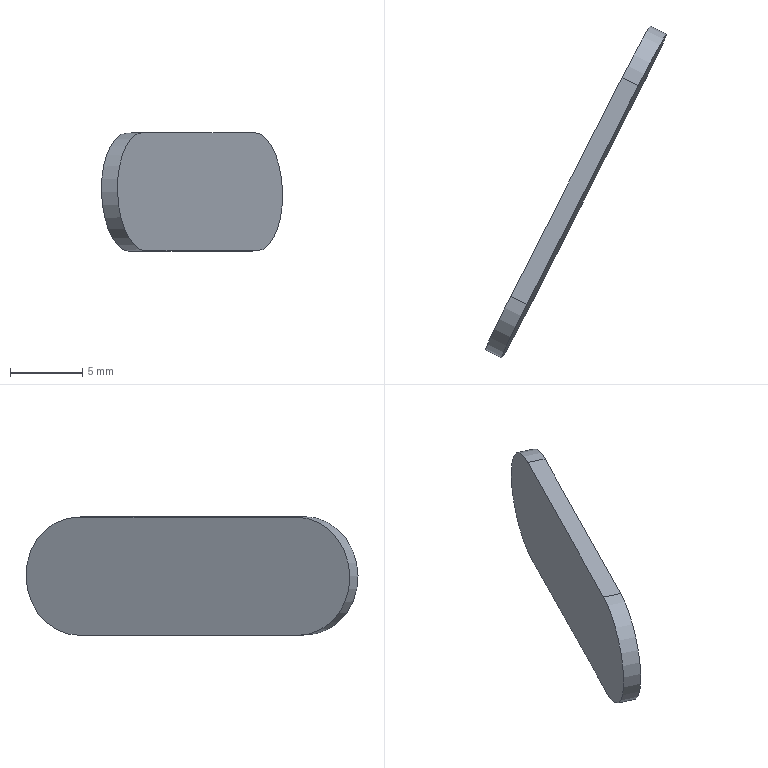Part | STEP file | 9805823280.1BPIECE_SOLIDE_FINALE_id1758_x_t | 1 solid | 6 faces | box 12.56 x 23.021 x 8.234 mm | volume 240.263 mm3 | plane 4 | cylinder 2 | commonest cylinder face diameters 8.2 x2
STEP:
#1=CARTESIAN_POINT('',(0.,0.,0.));
#2=DIRECTION('',(0.,0.,1.));
#3=DIRECTION('',(1.,0.,0.));
#4=AXIS2_PLACEMENT_3D('',#1,#2,#3);
#5=CARTESIAN_POINT('',(1096.718,-7.794,-24.025));
#6=VERTEX_POINT('',#5);
#7=CARTESIAN_POINT('',(1089.,-22.942,-24.025));
#8=VERTEX_POINT('',#7);
#9=CARTESIAN_POINT('',(1092.859,-15.368,-24.025));
#10=DIRECTION('',(-0.454,-0.891,0.));
#11=VECTOR('',#10,1.);
#12=LINE('',#9,#11);
#13=CARTESIAN_POINT('',(1077.019,-59.966,-230.062));
#14=DIRECTION('',(-0.8906,0.4538,-0.02975));
#15=DIRECTION('',(-0.02651,0.01351,0.9996));
#16=AXIS2_PLACEMENT_3D('',#13,#14,#15);
#17=PLANE('',#16);
#18=CARTESIAN_POINT('',(206.129,46.928));
#19=DIRECTION('',(0.000000001,-1.));
#20=VECTOR('',#19,1.);
#21=LINE('',#18,#20);
#22=(GEOMETRIC_REPRESENTATION_CONTEXT(2)PARAMETRIC_REPRESENTATION_CONTEXT()REPRESENTATION_CONTEXT('',''));
#23=DEFINITIONAL_REPRESENTATION('',(#21),#22);
#24=PCURVE('',#17,#23);
#25=CARTESIAN_POINT('',(1097.831,-8.362,-23.988));
#26=DIRECTION('',(0.02651,-0.01351,-0.9996));
#27=DIRECTION('',(0.454,0.891,0.));
#28=AXIS2_PLACEMENT_3D('',#25,#26,#27);
#29=PLANE('',#28);
#30=CARTESIAN_POINT('',(-8.5,-1.25));
#31=DIRECTION('',(-1.,0.));
#32=VECTOR('',#31,1.);
#33=LINE('',#30,#32);
#34=(GEOMETRIC_REPRESENTATION_CONTEXT(2)PARAMETRIC_REPRESENTATION_CONTEXT()REPRESENTATION_CONTEXT('',''));
#35=DEFINITIONAL_REPRESENTATION('',(#33),#34);
#36=PCURVE('',#29,#35);
#37=SURFACE_CURVE('',#12,(#24,#36),.PCURVE_S1.);
#38=EDGE_CURVE('',#6,#8,#37,.T.);
#39=ORIENTED_EDGE('',*,*,#38,.T.);
#40=CARTESIAN_POINT('',(1088.783,-22.831,-15.828));
#41=VERTEX_POINT('',#40);
#42=CARTESIAN_POINT('',(1088.892,-22.886,-19.927));
#43=DIRECTION('',(-0.8906,0.4538,-0.02975));
#44=DIRECTION('',(-0.02651,0.01351,0.9996));
#45=AXIS2_PLACEMENT_3D('',#42,#43,#44);
#46=CIRCLE('',#45,4.1);
#47=CARTESIAN_POINT('',(210.229,38.428));
#48=DIRECTION('',(1.,0.000000001));
#49=AXIS2_PLACEMENT_2D('',#47,#48);
#50=CIRCLE('',#49,4.1);
#51=(GEOMETRIC_REPRESENTATION_CONTEXT(2)PARAMETRIC_REPRESENTATION_CONTEXT()REPRESENTATION_CONTEXT('',''));
#52=DEFINITIONAL_REPRESENTATION('',(#50),#51);
#53=PCURVE('',#17,#52);
#54=CARTESIAN_POINT('',(1090.005,-23.453,-19.889));
#55=DIRECTION('',(0.8906,-0.4538,0.02975));
#56=DIRECTION('',(0.02651,-0.01351,-0.9996));
#57=AXIS2_PLACEMENT_3D('',#54,#55,#56);
#58=CYLINDRICAL_SURFACE('',#57,4.1);
#59=CARTESIAN_POINT('',(9.425,-1.25));
#60=DIRECTION('',(-1.,0.));
#61=VECTOR('',#60,1.);
#62=LINE('',#59,#61);
#63=(GEOMETRIC_REPRESENTATION_CONTEXT(2)PARAMETRIC_REPRESENTATION_CONTEXT()REPRESENTATION_CONTEXT('',''));
#64=DEFINITIONAL_REPRESENTATION('',(#62),#63);
#65=PCURVE('',#58,#64);
#66=SURFACE_CURVE('',#46,(#53,#65),.PCURVE_S1.);
#67=EDGE_CURVE('',#8,#41,#66,.T.);
#68=ORIENTED_EDGE('',*,*,#67,.T.);
#69=CARTESIAN_POINT('',(1096.501,-7.684,-15.828));
#70=VERTEX_POINT('',#69);
#71=CARTESIAN_POINT('',(1092.642,-15.257,-15.828));
#72=DIRECTION('',(0.454,0.891,0.));
#73=VECTOR('',#72,1.);
#74=LINE('',#71,#73);
#75=CARTESIAN_POINT('',(214.329,46.928));
#76=DIRECTION('',(-0.000000001,1.));
#77=VECTOR('',#76,1.);
#78=LINE('',#75,#77);
#79=(GEOMETRIC_REPRESENTATION_CONTEXT(2)PARAMETRIC_REPRESENTATION_CONTEXT()REPRESENTATION_CONTEXT('',''));
#80=DEFINITIONAL_REPRESENTATION('',(#78),#79);
#81=PCURVE('',#17,#80);
#82=CARTESIAN_POINT('',(1089.896,-23.398,-15.791));
#83=DIRECTION('',(-0.02651,0.01351,0.9996));
#84=DIRECTION('',(-0.454,-0.891,0.));
#85=AXIS2_PLACEMENT_3D('',#82,#83,#84);
#86=PLANE('',#85);
#87=CARTESIAN_POINT('',(-8.5,-1.25));
#88=DIRECTION('',(-1.,0.));
#89=VECTOR('',#88,1.);
#90=LINE('',#87,#89);
#91=(GEOMETRIC_REPRESENTATION_CONTEXT(2)PARAMETRIC_REPRESENTATION_CONTEXT()REPRESENTATION_CONTEXT('',''));
#92=DEFINITIONAL_REPRESENTATION('',(#90),#91);
#93=PCURVE('',#86,#92);
#94=SURFACE_CURVE('',#74,(#81,#93),.PCURVE_S1.);
#95=EDGE_CURVE('',#41,#70,#94,.T.);
#96=ORIENTED_EDGE('',*,*,#95,.T.);
#97=CARTESIAN_POINT('',(1096.609,-7.739,-19.927));
#98=DIRECTION('',(-0.8906,0.4538,-0.02975));
#99=DIRECTION('',(-0.02651,0.01351,0.9996));
#100=AXIS2_PLACEMENT_3D('',#97,#98,#99);
#101=CIRCLE('',#100,4.1);
#102=CARTESIAN_POINT('',(210.229,55.428));
#103=DIRECTION('',(1.,0.000000001));
#104=AXIS2_PLACEMENT_2D('',#102,#103);
#105=CIRCLE('',#104,4.1);
#106=(GEOMETRIC_REPRESENTATION_CONTEXT(2)PARAMETRIC_REPRESENTATION_CONTEXT()REPRESENTATION_CONTEXT('',''));
#107=DEFINITIONAL_REPRESENTATION('',(#105),#106);
#108=PCURVE('',#17,#107);
#109=CARTESIAN_POINT('',(1097.723,-8.306,-19.889));
#110=DIRECTION('',(0.8906,-0.4538,0.02975));
#111=DIRECTION('',(-0.02651,0.01351,0.9996));
#112=AXIS2_PLACEMENT_3D('',#109,#110,#111);
#113=CYLINDRICAL_SURFACE('',#112,4.1);
#114=CARTESIAN_POINT('',(6.283,-1.25));
#115=DIRECTION('',(-1.,0.));
#116=VECTOR('',#115,1.);
#117=LINE('',#114,#116);
#118=(GEOMETRIC_REPRESENTATION_CONTEXT(2)PARAMETRIC_REPRESENTATION_CONTEXT()REPRESENTATION_CONTEXT('',''));
#119=DEFINITIONAL_REPRESENTATION('',(#117),#118);
#120=PCURVE('',#113,#119);
#121=SURFACE_CURVE('',#101,(#108,#120),.PCURVE_S1.);
#122=EDGE_CURVE('',#70,#6,#121,.T.);
#123=ORIENTED_EDGE('',*,*,#122,.T.);
#124=EDGE_LOOP('',(#39,#68,#96,#123));
#125=FACE_BOUND('',#124,.T.);
#126=ADVANCED_FACE('',(#125),#17,.T.);
#127=CARTESIAN_POINT('',(1090.113,-23.509,-23.988));
#128=VERTEX_POINT('',#127);
#129=CARTESIAN_POINT('',(1090.113,-23.509,-23.988));
#130=DIRECTION('',(0.8906,-0.4538,0.02975));
#131=VECTOR('',#130,1.);
#132=LINE('',#129,#131);
#133=CARTESIAN_POINT('',(6.283,0.));
#134=DIRECTION('',(0.,1.));
#135=VECTOR('',#134,1.);
#136=LINE('',#133,#135);
#137=(GEOMETRIC_REPRESENTATION_CONTEXT(2)PARAMETRIC_REPRESENTATION_CONTEXT()REPRESENTATION_CONTEXT('',''));
#138=DEFINITIONAL_REPRESENTATION('',(#136),#137);
#139=PCURVE('',#58,#138);
#140=CARTESIAN_POINT('',(-17.,0.));
#141=DIRECTION('',(0.,1.));
#142=VECTOR('',#141,1.);
#143=LINE('',#140,#142);
#144=(GEOMETRIC_REPRESENTATION_CONTEXT(2)PARAMETRIC_REPRESENTATION_CONTEXT()REPRESENTATION_CONTEXT('',''));
#145=DEFINITIONAL_REPRESENTATION('',(#143),#144);
#146=PCURVE('',#29,#145);
#147=SURFACE_CURVE('',#132,(#139,#146),.PCURVE_S1.);
#148=EDGE_CURVE('',#8,#128,#147,.T.);
#149=ORIENTED_EDGE('',*,*,#148,.T.);
#150=CARTESIAN_POINT('',(1089.896,-23.398,-15.791));
#151=VERTEX_POINT('',#150);
#152=CARTESIAN_POINT('',(1090.005,-23.453,-19.889));
#153=DIRECTION('',(-0.8906,0.4538,-0.02975));
#154=DIRECTION('',(-0.02651,0.01351,0.9996));
#155=AXIS2_PLACEMENT_3D('',#152,#153,#154);
#156=CIRCLE('',#155,4.1);
#157=CARTESIAN_POINT('',(9.425,0.));
#158=DIRECTION('',(-1.,0.));
#159=VECTOR('',#158,1.);
#160=LINE('',#157,#159);
#161=(GEOMETRIC_REPRESENTATION_CONTEXT(2)PARAMETRIC_REPRESENTATION_CONTEXT()REPRESENTATION_CONTEXT('',''));
#162=DEFINITIONAL_REPRESENTATION('',(#160),#161);
#163=PCURVE('',#58,#162);
#164=CARTESIAN_POINT('',(1078.132,-60.533,-230.025));
#165=DIRECTION('',(-0.8906,0.4538,-0.02975));
#166=DIRECTION('',(-0.02651,0.01351,0.9996));
#167=AXIS2_PLACEMENT_3D('',#164,#165,#166);
#168=PLANE('',#167);
#169=CARTESIAN_POINT('',(210.229,38.428));
#170=DIRECTION('',(1.,0.000000001));
#171=AXIS2_PLACEMENT_2D('',#169,#170);
#172=CIRCLE('',#171,4.1);
#173=(GEOMETRIC_REPRESENTATION_CONTEXT(2)PARAMETRIC_REPRESENTATION_CONTEXT()REPRESENTATION_CONTEXT('',''));
#174=DEFINITIONAL_REPRESENTATION('',(#172),#173);
#175=PCURVE('',#168,#174);
#176=SURFACE_CURVE('',#156,(#163,#175),.PCURVE_S1.);
#177=EDGE_CURVE('',#128,#151,#176,.T.);
#178=ORIENTED_EDGE('',*,*,#177,.T.);
#179=CARTESIAN_POINT('',(1089.896,-23.398,-15.791));
#180=DIRECTION('',(0.8906,-0.4538,0.02975));
#181=VECTOR('',#180,1.);
#182=LINE('',#179,#181);
#183=CARTESIAN_POINT('',(3.142,0.));
#184=DIRECTION('',(0.,1.));
#185=VECTOR('',#184,1.);
#186=LINE('',#183,#185);
#187=(GEOMETRIC_REPRESENTATION_CONTEXT(2)PARAMETRIC_REPRESENTATION_CONTEXT()REPRESENTATION_CONTEXT('',''));
#188=DEFINITIONAL_REPRESENTATION('',(#186),#187);
#189=PCURVE('',#58,#188);
#190=CARTESIAN_POINT('',(0.,0.));
#191=DIRECTION('',(0.,1.));
#192=VECTOR('',#191,1.);
#193=LINE('',#190,#192);
#194=(GEOMETRIC_REPRESENTATION_CONTEXT(2)PARAMETRIC_REPRESENTATION_CONTEXT()REPRESENTATION_CONTEXT('',''));
#195=DEFINITIONAL_REPRESENTATION('',(#193),#194);
#196=PCURVE('',#86,#195);
#197=SURFACE_CURVE('',#182,(#189,#196),.PCURVE_S1.);
#198=EDGE_CURVE('',#41,#151,#197,.T.);
#199=ORIENTED_EDGE('',*,*,#198,.F.);
#200=ORIENTED_EDGE('',*,*,#67,.F.);
#201=EDGE_LOOP('',(#149,#178,#199,#200));
#202=FACE_BOUND('',#201,.T.);
#203=ADVANCED_FACE('',(#202),#58,.T.);
#204=CARTESIAN_POINT('',(1097.831,-8.362,-23.988));
#205=VERTEX_POINT('',#204);
#206=CARTESIAN_POINT('',(1097.275,-8.078,-24.006));
#207=DIRECTION('',(0.8906,-0.4538,0.02975));
#208=VECTOR('',#207,1.);
#209=LINE('',#206,#208);
#210=CARTESIAN_POINT('',(0.,-0.625));
#211=DIRECTION('',(0.,1.));
#212=VECTOR('',#211,1.);
#213=LINE('',#210,#212);
#214=(GEOMETRIC_REPRESENTATION_CONTEXT(2)PARAMETRIC_REPRESENTATION_CONTEXT()REPRESENTATION_CONTEXT('',''));
#215=DEFINITIONAL_REPRESENTATION('',(#213),#214);
#216=PCURVE('',#29,#215);
#217=CARTESIAN_POINT('',(3.142,-0.625));
#218=DIRECTION('',(0.,1.));
#219=VECTOR('',#218,1.);
#220=LINE('',#217,#219);
#221=(GEOMETRIC_REPRESENTATION_CONTEXT(2)PARAMETRIC_REPRESENTATION_CONTEXT()REPRESENTATION_CONTEXT('',''));
#222=DEFINITIONAL_REPRESENTATION('',(#220),#221);
#223=PCURVE('',#113,#222);
#224=SURFACE_CURVE('',#209,(#216,#223),.PCURVE_S1.);
#225=EDGE_CURVE('',#6,#205,#224,.T.);
#226=ORIENTED_EDGE('',*,*,#225,.T.);
#227=CARTESIAN_POINT('',(1093.972,-15.935,-23.988));
#228=DIRECTION('',(-0.454,-0.891,0.));
#229=VECTOR('',#228,1.);
#230=LINE('',#227,#229);
#231=CARTESIAN_POINT('',(-8.5,0.));
#232=DIRECTION('',(-1.,0.));
#233=VECTOR('',#232,1.);
#234=LINE('',#231,#233);
#235=(GEOMETRIC_REPRESENTATION_CONTEXT(2)PARAMETRIC_REPRESENTATION_CONTEXT()REPRESENTATION_CONTEXT('',''));
#236=DEFINITIONAL_REPRESENTATION('',(#234),#235);
#237=PCURVE('',#29,#236);
#238=CARTESIAN_POINT('',(206.129,46.928));
#239=DIRECTION('',(0.000000001,-1.));
#240=VECTOR('',#239,1.);
#241=LINE('',#238,#240);
#242=(GEOMETRIC_REPRESENTATION_CONTEXT(2)PARAMETRIC_REPRESENTATION_CONTEXT()REPRESENTATION_CONTEXT('',''));
#243=DEFINITIONAL_REPRESENTATION('',(#241),#242);
#244=PCURVE('',#168,#243);
#245=SURFACE_CURVE('',#230,(#237,#244),.PCURVE_S1.);
#246=EDGE_CURVE('',#205,#128,#245,.T.);
#247=ORIENTED_EDGE('',*,*,#246,.T.);
#248=ORIENTED_EDGE('',*,*,#148,.F.);
#249=ORIENTED_EDGE('',*,*,#38,.F.);
#250=EDGE_LOOP('',(#226,#247,#248,#249));
#251=FACE_BOUND('',#250,.T.);
#252=ADVANCED_FACE('',(#251),#29,.T.);
#253=CARTESIAN_POINT('',(1097.614,-8.251,-15.791));
#254=VERTEX_POINT('',#253);
#255=CARTESIAN_POINT('',(1097.057,-7.967,-15.81));
#256=DIRECTION('',(0.8906,-0.4538,0.02975));
#257=VECTOR('',#256,1.);
#258=LINE('',#255,#257);
#259=CARTESIAN_POINT('',(6.283,-0.625));
#260=DIRECTION('',(0.,1.));
#261=VECTOR('',#260,1.);
#262=LINE('',#259,#261);
#263=(GEOMETRIC_REPRESENTATION_CONTEXT(2)PARAMETRIC_REPRESENTATION_CONTEXT()REPRESENTATION_CONTEXT('',''));
#264=DEFINITIONAL_REPRESENTATION('',(#262),#263);
#265=PCURVE('',#113,#264);
#266=CARTESIAN_POINT('',(-17.,-0.625));
#267=DIRECTION('',(0.,1.));
#268=VECTOR('',#267,1.);
#269=LINE('',#266,#268);
#270=(GEOMETRIC_REPRESENTATION_CONTEXT(2)PARAMETRIC_REPRESENTATION_CONTEXT()REPRESENTATION_CONTEXT('',''));
#271=DEFINITIONAL_REPRESENTATION('',(#269),#270);
#272=PCURVE('',#86,#271);
#273=SURFACE_CURVE('',#258,(#265,#272),.PCURVE_S1.);
#274=EDGE_CURVE('',#70,#254,#273,.T.);
#275=ORIENTED_EDGE('',*,*,#274,.T.);
#276=CARTESIAN_POINT('',(1097.723,-8.306,-19.889));
#277=DIRECTION('',(-0.8906,0.4538,-0.02975));
#278=DIRECTION('',(-0.02651,0.01351,0.9996));
#279=AXIS2_PLACEMENT_3D('',#276,#277,#278);
#280=CIRCLE('',#279,4.1);
#281=CARTESIAN_POINT('',(6.283,0.));
#282=DIRECTION('',(-1.,0.));
#283=VECTOR('',#282,1.);
#284=LINE('',#281,#283);
#285=(GEOMETRIC_REPRESENTATION_CONTEXT(2)PARAMETRIC_REPRESENTATION_CONTEXT()REPRESENTATION_CONTEXT('',''));
#286=DEFINITIONAL_REPRESENTATION('',(#284),#285);
#287=PCURVE('',#113,#286);
#288=CARTESIAN_POINT('',(210.229,55.428));
#289=DIRECTION('',(1.,0.000000001));
#290=AXIS2_PLACEMENT_2D('',#288,#289);
#291=CIRCLE('',#290,4.1);
#292=(GEOMETRIC_REPRESENTATION_CONTEXT(2)PARAMETRIC_REPRESENTATION_CONTEXT()REPRESENTATION_CONTEXT('',''));
#293=DEFINITIONAL_REPRESENTATION('',(#291),#292);
#294=PCURVE('',#168,#293);
#295=SURFACE_CURVE('',#280,(#287,#294),.PCURVE_S1.);
#296=EDGE_CURVE('',#254,#205,#295,.T.);
#297=ORIENTED_EDGE('',*,*,#296,.T.);
#298=ORIENTED_EDGE('',*,*,#225,.F.);
#299=ORIENTED_EDGE('',*,*,#122,.F.);
#300=EDGE_LOOP('',(#275,#297,#298,#299));
#301=FACE_BOUND('',#300,.T.);
#302=ADVANCED_FACE('',(#301),#113,.T.);
#303=ORIENTED_EDGE('',*,*,#198,.T.);
#304=CARTESIAN_POINT('',(1093.755,-15.824,-15.791));
#305=DIRECTION('',(0.454,0.891,0.));
#306=VECTOR('',#305,1.);
#307=LINE('',#304,#306);
#308=CARTESIAN_POINT('',(-8.5,0.));
#309=DIRECTION('',(-1.,0.));
#310=VECTOR('',#309,1.);
#311=LINE('',#308,#310);
#312=(GEOMETRIC_REPRESENTATION_CONTEXT(2)PARAMETRIC_REPRESENTATION_CONTEXT()REPRESENTATION_CONTEXT('',''));
#313=DEFINITIONAL_REPRESENTATION('',(#311),#312);
#314=PCURVE('',#86,#313);
#315=CARTESIAN_POINT('',(214.329,46.928));
#316=DIRECTION('',(-0.000000001,1.));
#317=VECTOR('',#316,1.);
#318=LINE('',#315,#317);
#319=(GEOMETRIC_REPRESENTATION_CONTEXT(2)PARAMETRIC_REPRESENTATION_CONTEXT()REPRESENTATION_CONTEXT('',''));
#320=DEFINITIONAL_REPRESENTATION('',(#318),#319);
#321=PCURVE('',#168,#320);
#322=SURFACE_CURVE('',#307,(#314,#321),.PCURVE_S1.);
#323=EDGE_CURVE('',#151,#254,#322,.T.);
#324=ORIENTED_EDGE('',*,*,#323,.T.);
#325=ORIENTED_EDGE('',*,*,#274,.F.);
#326=ORIENTED_EDGE('',*,*,#95,.F.);
#327=EDGE_LOOP('',(#303,#324,#325,#326));
#328=FACE_BOUND('',#327,.T.);
#329=ADVANCED_FACE('',(#328),#86,.T.);
#330=ORIENTED_EDGE('',*,*,#296,.T.);
#331=ORIENTED_EDGE('',*,*,#246,.T.);
#332=ORIENTED_EDGE('',*,*,#177,.T.);
#333=ORIENTED_EDGE('',*,*,#323,.T.);
#334=EDGE_LOOP('',(#330,#331,#332,#333));
#335=FACE_BOUND('',#334,.F.);
#336=ADVANCED_FACE('',(#335),#168,.F.);
#337=CLOSED_SHELL('',(#126,#203,#252,#302,#329,#336));
#338=MANIFOLD_SOLID_BREP('',#337);
#339=(LENGTH_UNIT()NAMED_UNIT(*)SI_UNIT(.MILLI.,.METRE.));
#340=UNCERTAINTY_MEASURE_WITH_UNIT(LENGTH_MEASURE(0.000001),#339,'','');
#341=(NAMED_UNIT(*)PLANE_ANGLE_UNIT()SI_UNIT($,.RADIAN.));
#342=(NAMED_UNIT(*)SI_UNIT($,.STERADIAN.)SOLID_ANGLE_UNIT());
#343=(GEOMETRIC_REPRESENTATION_CONTEXT(3)GLOBAL_UNCERTAINTY_ASSIGNED_CONTEXT((#340))GLOBAL_UNIT_ASSIGNED_CONTEXT((#339,#341,#342))REPRESENTATION_CONTEXT('',''));
#344=ADVANCED_BREP_SHAPE_REPRESENTATION('',(#4,#338),#343);